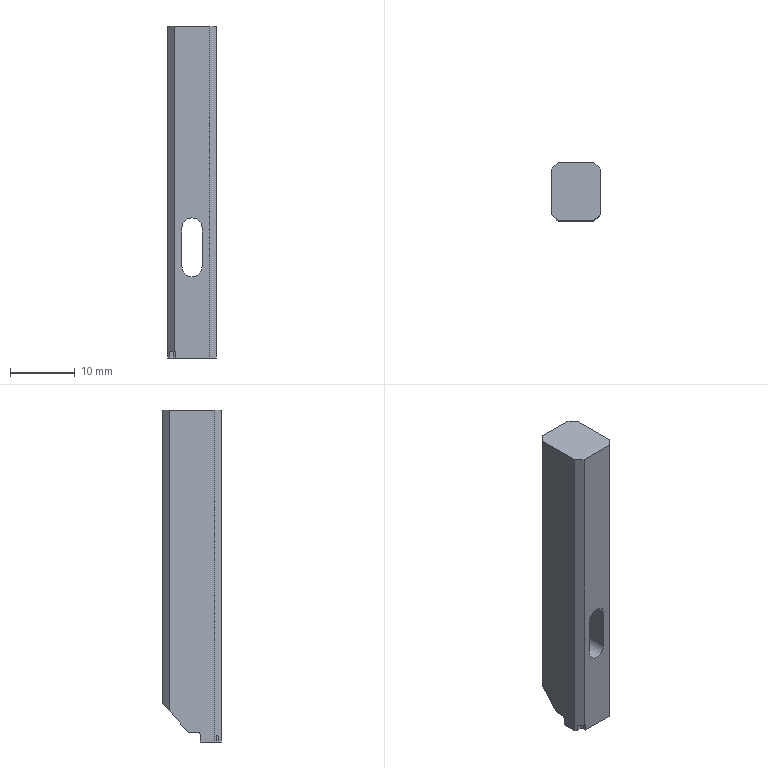Part | STEP file | 03-12 trimming upper-left blade | 1 solid | 23 faces | box 7.5 x 9 x 51.3 mm | volume 2999 mm3 | plane 18 | cylinder 5 | commonest cylinder face diameters 3.1 x3 0.7 x1 1 x1
STEP:
#1=CARTESIAN_POINT('',(3.13,-4.5,21.65));
#2=VERTEX_POINT('',#1);
#3=CARTESIAN_POINT('',(4.68,-4.5,20.1));
#4=VERTEX_POINT('',#3);
#5=CARTESIAN_POINT('',(3.13,-4.5,20.1));
#6=DIRECTION('',(0.,1.,0.));
#7=DIRECTION('',(0.,0.,1.));
#8=AXIS2_PLACEMENT_3D('',#5,#6,#7);
#9=CIRCLE('',#8,1.55);
#10=EDGE_CURVE('',#2,#4,#9,.T.);
#11=ORIENTED_EDGE('',*,*,#10,.F.);
#12=CARTESIAN_POINT('',(3.13,4.5,21.65));
#13=VERTEX_POINT('',#12);
#14=CARTESIAN_POINT('',(3.13,-8.5,21.65));
#15=DIRECTION('',(0.,1.,0.));
#16=VECTOR('',#15,1000.);
#17=LINE('',#14,#16);
#18=EDGE_CURVE('',#2,#13,#17,.T.);
#19=ORIENTED_EDGE('',*,*,#18,.T.);
#20=CARTESIAN_POINT('',(4.68,4.5,20.1));
#21=VERTEX_POINT('',#20);
#22=CARTESIAN_POINT('',(3.13,4.5,20.1));
#23=DIRECTION('',(0.,1.,0.));
#24=DIRECTION('',(0.,0.,1.));
#25=AXIS2_PLACEMENT_3D('',#22,#23,#24);
#26=CIRCLE('',#25,1.55);
#27=EDGE_CURVE('',#13,#21,#26,.T.);
#28=ORIENTED_EDGE('',*,*,#27,.T.);
#29=CARTESIAN_POINT('',(4.68,-8.5,20.1));
#30=DIRECTION('',(0.,1.,0.));
#31=VECTOR('',#30,1000.);
#32=LINE('',#29,#31);
#33=EDGE_CURVE('',#4,#21,#32,.T.);
#34=ORIENTED_EDGE('',*,*,#33,.F.);
#35=EDGE_LOOP('',(#11,#19,#28,#34));
#36=FACE_OUTER_BOUND('',#35,.T.);
#37=CARTESIAN_POINT('',(3.13,-8.5,20.1));
#38=DIRECTION('',(0.,1.,0.));
#39=DIRECTION('',(0.,0.,1.));
#40=AXIS2_PLACEMENT_3D('',#37,#38,#39);
#41=CYLINDRICAL_SURFACE('',#40,1.55);
#42=ADVANCED_FACE('',(#36),#41,.F.);
#43=CARTESIAN_POINT('',(4.68,4.5,14.1));
#44=VERTEX_POINT('',#43);
#45=CARTESIAN_POINT('',(4.68,4.5,20.1));
#46=DIRECTION('',(0.,0.,-1.));
#47=VECTOR('',#46,1000.);
#48=LINE('',#45,#47);
#49=EDGE_CURVE('',#21,#44,#48,.T.);
#50=ORIENTED_EDGE('',*,*,#49,.F.);
#51=ORIENTED_EDGE('',*,*,#27,.F.);
#52=CARTESIAN_POINT('',(1.58,4.5,20.1));
#53=VERTEX_POINT('',#52);
#54=CARTESIAN_POINT('',(3.13,4.5,20.1));
#55=DIRECTION('',(0.,1.,0.));
#56=DIRECTION('',(0.,0.,1.));
#57=AXIS2_PLACEMENT_3D('',#54,#55,#56);
#58=CIRCLE('',#57,1.55);
#59=EDGE_CURVE('',#53,#13,#58,.T.);
#60=ORIENTED_EDGE('',*,*,#59,.F.);
#61=CARTESIAN_POINT('',(1.58,4.5,14.1));
#62=VERTEX_POINT('',#61);
#63=CARTESIAN_POINT('',(1.58,4.5,20.1));
#64=DIRECTION('',(0.,0.,1.));
#65=VECTOR('',#64,1000.);
#66=LINE('',#63,#65);
#67=EDGE_CURVE('',#62,#53,#66,.T.);
#68=ORIENTED_EDGE('',*,*,#67,.F.);
#69=CARTESIAN_POINT('',(3.13,4.5,14.1));
#70=DIRECTION('',(0.,1.,0.));
#71=DIRECTION('',(0.,0.,1.));
#72=AXIS2_PLACEMENT_3D('',#69,#70,#71);
#73=CIRCLE('',#72,1.55);
#74=EDGE_CURVE('',#44,#62,#73,.T.);
#75=ORIENTED_EDGE('',*,*,#74,.F.);
#76=EDGE_LOOP('',(#50,#51,#60,#68,#75));
#77=FACE_BOUND('',#76,.T.);
#78=CARTESIAN_POINT('',(5.88,4.5,6.));
#79=VERTEX_POINT('',#78);
#80=CARTESIAN_POINT('',(0.3804,4.5,6.));
#81=VERTEX_POINT('',#80);
#82=CARTESIAN_POINT('',(7.38,4.5,6.));
#83=DIRECTION('',(-1.,0.,0.));
#84=VECTOR('',#83,1000.);
#85=LINE('',#82,#84);
#86=EDGE_CURVE('',#79,#81,#85,.T.);
#87=ORIENTED_EDGE('',*,*,#86,.T.);
#88=CARTESIAN_POINT('',(0.3804,4.5,51.3));
#89=VERTEX_POINT('',#88);
#90=CARTESIAN_POINT('',(0.3804,4.5,51.3));
#91=DIRECTION('',(0.,0.,1.));
#92=VECTOR('',#91,1000.);
#93=LINE('',#90,#92);
#94=EDGE_CURVE('',#81,#89,#93,.T.);
#95=ORIENTED_EDGE('',*,*,#94,.T.);
#96=CARTESIAN_POINT('',(5.88,4.5,51.3));
#97=VERTEX_POINT('',#96);
#98=CARTESIAN_POINT('',(-6.,4.5,51.3));
#99=DIRECTION('',(-1.,0.,0.));
#100=VECTOR('',#99,1000.);
#101=LINE('',#98,#100);
#102=EDGE_CURVE('',#97,#89,#101,.T.);
#103=ORIENTED_EDGE('',*,*,#102,.F.);
#104=CARTESIAN_POINT('',(5.88,4.5,51.3));
#105=DIRECTION('',(0.,0.,-1.));
#106=VECTOR('',#105,1000.);
#107=LINE('',#104,#106);
#108=EDGE_CURVE('',#97,#79,#107,.T.);
#109=ORIENTED_EDGE('',*,*,#108,.T.);
#110=EDGE_LOOP('',(#87,#95,#103,#109));
#111=FACE_OUTER_BOUND('',#110,.T.);
#112=CARTESIAN_POINT('',(-6.,4.5,51.3));
#113=DIRECTION('',(0.,-1.,0.));
#114=DIRECTION('',(0.,0.,-1.));
#115=AXIS2_PLACEMENT_3D('',#112,#113,#114);
#116=PLANE('',#115);
#117=ADVANCED_FACE('',(#77,#111),#116,.F.);
#118=CARTESIAN_POINT('',(1.58,-4.5,14.1));
#119=VERTEX_POINT('',#118);
#120=CARTESIAN_POINT('',(1.58,-4.5,20.1));
#121=VERTEX_POINT('',#120);
#122=CARTESIAN_POINT('',(1.58,-4.5,51.3));
#123=DIRECTION('',(0.,0.,1.));
#124=VECTOR('',#123,1000.);
#125=LINE('',#122,#124);
#126=EDGE_CURVE('',#119,#121,#125,.T.);
#127=ORIENTED_EDGE('',*,*,#126,.T.);
#128=CARTESIAN_POINT('',(3.13,-4.5,20.1));
#129=DIRECTION('',(0.,1.,0.));
#130=DIRECTION('',(0.,0.,1.));
#131=AXIS2_PLACEMENT_3D('',#128,#129,#130);
#132=CIRCLE('',#131,1.55);
#133=EDGE_CURVE('',#121,#2,#132,.T.);
#134=ORIENTED_EDGE('',*,*,#133,.T.);
#135=ORIENTED_EDGE('',*,*,#10,.T.);
#136=CARTESIAN_POINT('',(4.68,-4.5,14.1));
#137=VERTEX_POINT('',#136);
#138=CARTESIAN_POINT('',(4.68,-4.5,51.3));
#139=DIRECTION('',(0.,0.,-1.));
#140=VECTOR('',#139,1000.);
#141=LINE('',#138,#140);
#142=EDGE_CURVE('',#4,#137,#141,.T.);
#143=ORIENTED_EDGE('',*,*,#142,.T.);
#144=CARTESIAN_POINT('',(3.13,-4.5,14.1));
#145=DIRECTION('',(0.,1.,0.));
#146=DIRECTION('',(0.,0.,1.));
#147=AXIS2_PLACEMENT_3D('',#144,#145,#146);
#148=CIRCLE('',#147,1.55);
#149=EDGE_CURVE('',#137,#119,#148,.T.);
#150=ORIENTED_EDGE('',*,*,#149,.T.);
#151=EDGE_LOOP('',(#127,#134,#135,#143,#150));
#152=FACE_BOUND('',#151,.T.);
#153=CARTESIAN_POINT('',(0.6304,-4.5,1.));
#154=VERTEX_POINT('',#153);
#155=CARTESIAN_POINT('',(0.3804,-4.5,1.));
#156=VERTEX_POINT('',#155);
#157=CARTESIAN_POINT('',(-6.,-4.5,1.));
#158=DIRECTION('',(-1.,0.,0.));
#159=VECTOR('',#158,1000.);
#160=LINE('',#157,#159);
#161=EDGE_CURVE('',#154,#156,#160,.T.);
#162=ORIENTED_EDGE('',*,*,#161,.F.);
#163=CARTESIAN_POINT('',(0.6304,-4.5,0.));
#164=VERTEX_POINT('',#163);
#165=CARTESIAN_POINT('',(0.6304,-4.5,51.3));
#166=DIRECTION('',(0.,0.,-1.));
#167=VECTOR('',#166,1000.);
#168=LINE('',#165,#167);
#169=EDGE_CURVE('',#154,#164,#168,.T.);
#170=ORIENTED_EDGE('',*,*,#169,.T.);
#171=CARTESIAN_POINT('',(5.88,-4.5,0.));
#172=VERTEX_POINT('',#171);
#173=CARTESIAN_POINT('',(-6.,-4.5,0.));
#174=DIRECTION('',(1.,0.,0.));
#175=VECTOR('',#174,1000.);
#176=LINE('',#173,#175);
#177=EDGE_CURVE('',#164,#172,#176,.T.);
#178=ORIENTED_EDGE('',*,*,#177,.T.);
#179=CARTESIAN_POINT('',(5.88,-4.5,51.3));
#180=VERTEX_POINT('',#179);
#181=CARTESIAN_POINT('',(5.88,-4.5,51.3));
#182=DIRECTION('',(0.,0.,1.));
#183=VECTOR('',#182,1000.);
#184=LINE('',#181,#183);
#185=EDGE_CURVE('',#172,#180,#184,.T.);
#186=ORIENTED_EDGE('',*,*,#185,.T.);
#187=CARTESIAN_POINT('',(0.3804,-4.5,51.3));
#188=VERTEX_POINT('',#187);
#189=CARTESIAN_POINT('',(-6.,-4.5,51.3));
#190=DIRECTION('',(1.,0.,0.));
#191=VECTOR('',#190,1000.);
#192=LINE('',#189,#191);
#193=EDGE_CURVE('',#188,#180,#192,.T.);
#194=ORIENTED_EDGE('',*,*,#193,.F.);
#195=CARTESIAN_POINT('',(0.3804,-4.5,51.3));
#196=DIRECTION('',(0.,0.,-1.));
#197=VECTOR('',#196,1000.);
#198=LINE('',#195,#197);
#199=EDGE_CURVE('',#188,#156,#198,.T.);
#200=ORIENTED_EDGE('',*,*,#199,.T.);
#201=EDGE_LOOP('',(#162,#170,#178,#186,#194,#200));
#202=FACE_OUTER_BOUND('',#201,.T.);
#203=CARTESIAN_POINT('',(-6.,-4.5,51.3));
#204=DIRECTION('',(0.,1.,0.));
#205=DIRECTION('',(0.,0.,1.));
#206=AXIS2_PLACEMENT_3D('',#203,#204,#205);
#207=PLANE('',#206);
#208=ADVANCED_FACE('',(#152,#202),#207,.F.);
#209=CARTESIAN_POINT('',(-0.6196,-3.5,51.3));
#210=VERTEX_POINT('',#209);
#211=CARTESIAN_POINT('',(-0.6196,3.5,51.3));
#212=VERTEX_POINT('',#211);
#213=CARTESIAN_POINT('',(-0.6196,-4.5,51.3));
#214=DIRECTION('',(0.,1.,0.));
#215=VECTOR('',#214,1000.);
#216=LINE('',#213,#215);
#217=EDGE_CURVE('',#210,#212,#216,.T.);
#218=ORIENTED_EDGE('',*,*,#217,.F.);
#219=CARTESIAN_POINT('',(3.19,-7.31,51.3));
#220=DIRECTION('',(0.7071,-0.7071,0.));
#221=VECTOR('',#220,1000.);
#222=LINE('',#219,#221);
#223=EDGE_CURVE('',#210,#188,#222,.T.);
#224=ORIENTED_EDGE('',*,*,#223,.T.);
#225=ORIENTED_EDGE('',*,*,#193,.T.);
#226=CARTESIAN_POINT('',(6.88,-3.5,51.3));
#227=VERTEX_POINT('',#226);
#228=CARTESIAN_POINT('',(5.94,-4.44,51.3));
#229=DIRECTION('',(0.7071,0.7071,0.));
#230=VECTOR('',#229,1000.);
#231=LINE('',#228,#230);
#232=EDGE_CURVE('',#180,#227,#231,.T.);
#233=ORIENTED_EDGE('',*,*,#232,.T.);
#234=CARTESIAN_POINT('',(6.88,3.5,51.3));
#235=VERTEX_POINT('',#234);
#236=CARTESIAN_POINT('',(6.88,-4.5,51.3));
#237=DIRECTION('',(0.,-1.,0.));
#238=VECTOR('',#237,1000.);
#239=LINE('',#236,#238);
#240=EDGE_CURVE('',#235,#227,#239,.T.);
#241=ORIENTED_EDGE('',*,*,#240,.F.);
#242=CARTESIAN_POINT('',(10.44,-0.05981,51.3));
#243=DIRECTION('',(-0.7071,0.7071,0.));
#244=VECTOR('',#243,1000.);
#245=LINE('',#242,#244);
#246=EDGE_CURVE('',#235,#97,#245,.T.);
#247=ORIENTED_EDGE('',*,*,#246,.T.);
#248=ORIENTED_EDGE('',*,*,#102,.T.);
#249=CARTESIAN_POINT('',(-1.31,2.81,51.3));
#250=DIRECTION('',(-0.7071,-0.7071,0.));
#251=VECTOR('',#250,1000.);
#252=LINE('',#249,#251);
#253=EDGE_CURVE('',#89,#212,#252,.T.);
#254=ORIENTED_EDGE('',*,*,#253,.T.);
#255=EDGE_LOOP('',(#218,#224,#225,#233,#241,#247,#248,#254));
#256=FACE_OUTER_BOUND('',#255,.T.);
#257=CARTESIAN_POINT('',(6.,-4.5,51.3));
#258=DIRECTION('',(0.,0.,1.));
#259=DIRECTION('',(1.,0.,0.));
#260=AXIS2_PLACEMENT_3D('',#257,#258,#259);
#261=PLANE('',#260);
#262=ADVANCED_FACE('',(#256),#261,.T.);
#263=CARTESIAN_POINT('',(0.2804,-3.75,0.));
#264=VERTEX_POINT('',#263);
#265=CARTESIAN_POINT('',(0.6304,-4.1,0.));
#266=VERTEX_POINT('',#265);
#267=CARTESIAN_POINT('',(0.2804,-4.1,0.));
#268=DIRECTION('',(0.,0.,-1.));
#269=DIRECTION('',(-1.,0.,0.));
#270=AXIS2_PLACEMENT_3D('',#267,#268,#269);
#271=CIRCLE('',#270,0.35);
#272=EDGE_CURVE('',#264,#266,#271,.T.);
#273=ORIENTED_EDGE('',*,*,#272,.F.);
#274=CARTESIAN_POINT('',(-0.3696,-3.75,0.));
#275=VERTEX_POINT('',#274);
#276=CARTESIAN_POINT('',(0.2804,-3.75,0.));
#277=DIRECTION('',(1.,0.,0.));
#278=VECTOR('',#277,1000.);
#279=LINE('',#276,#278);
#280=EDGE_CURVE('',#275,#264,#279,.T.);
#281=ORIENTED_EDGE('',*,*,#280,.F.);
#282=CARTESIAN_POINT('',(-0.6196,-3.5,0.));
#283=VERTEX_POINT('',#282);
#284=CARTESIAN_POINT('',(0.3804,-4.5,0.));
#285=DIRECTION('',(-0.7071,0.7071,0.));
#286=VECTOR('',#285,1000.);
#287=LINE('',#284,#286);
#288=EDGE_CURVE('',#275,#283,#287,.T.);
#289=ORIENTED_EDGE('',*,*,#288,.T.);
#290=CARTESIAN_POINT('',(-0.6196,-1.3,0.));
#291=VERTEX_POINT('',#290);
#292=CARTESIAN_POINT('',(-0.6196,4.5,0.));
#293=DIRECTION('',(0.,-1.,0.));
#294=VECTOR('',#293,1000.);
#295=LINE('',#292,#294);
#296=EDGE_CURVE('',#291,#283,#295,.T.);
#297=ORIENTED_EDGE('',*,*,#296,.F.);
#298=CARTESIAN_POINT('',(6.88,-1.3,0.));
#299=VERTEX_POINT('',#298);
#300=CARTESIAN_POINT('',(6.,-1.3,0.));
#301=DIRECTION('',(1.,0.,0.));
#302=VECTOR('',#301,1000.);
#303=LINE('',#300,#302);
#304=EDGE_CURVE('',#291,#299,#303,.T.);
#305=ORIENTED_EDGE('',*,*,#304,.T.);
#306=CARTESIAN_POINT('',(6.88,-3.5,0.));
#307=VERTEX_POINT('',#306);
#308=CARTESIAN_POINT('',(6.88,4.815,0.));
#309=DIRECTION('',(0.,1.,0.));
#310=VECTOR('',#309,1000.);
#311=LINE('',#308,#310);
#312=EDGE_CURVE('',#307,#299,#311,.T.);
#313=ORIENTED_EDGE('',*,*,#312,.F.);
#314=CARTESIAN_POINT('',(5.88,-4.5,0.));
#315=DIRECTION('',(-0.7071,-0.7071,0.));
#316=VECTOR('',#315,1000.);
#317=LINE('',#314,#316);
#318=EDGE_CURVE('',#307,#172,#317,.T.);
#319=ORIENTED_EDGE('',*,*,#318,.T.);
#320=ORIENTED_EDGE('',*,*,#177,.F.);
#321=CARTESIAN_POINT('',(0.6304,-4.1,0.));
#322=DIRECTION('',(0.,-1.,0.));
#323=VECTOR('',#322,1000.);
#324=LINE('',#321,#323);
#325=EDGE_CURVE('',#266,#164,#324,.T.);
#326=ORIENTED_EDGE('',*,*,#325,.F.);
#327=EDGE_LOOP('',(#273,#281,#289,#297,#305,#313,#319,#320,#326));
#328=FACE_OUTER_BOUND('',#327,.T.);
#329=CARTESIAN_POINT('',(6.,-4.5,0.));
#330=DIRECTION('',(0.,0.,1.));
#331=DIRECTION('',(1.,0.,0.));
#332=AXIS2_PLACEMENT_3D('',#329,#330,#331);
#333=PLANE('',#332);
#334=ADVANCED_FACE('',(#328),#333,.F.);
#335=ORIENTED_EDGE('',*,*,#296,.T.);
#336=CARTESIAN_POINT('',(-0.6196,-3.5,6.));
#337=DIRECTION('',(0.,0.,1.));
#338=VECTOR('',#337,1000.);
#339=LINE('',#336,#338);
#340=EDGE_CURVE('',#283,#210,#339,.T.);
#341=ORIENTED_EDGE('',*,*,#340,.T.);
#342=ORIENTED_EDGE('',*,*,#217,.T.);
#343=CARTESIAN_POINT('',(-0.6196,3.5,4.846));
#344=VERTEX_POINT('',#343);
#345=CARTESIAN_POINT('',(-0.6196,3.5,6.));
#346=DIRECTION('',(0.,0.,-1.));
#347=VECTOR('',#346,1000.);
#348=LINE('',#345,#347);
#349=EDGE_CURVE('',#212,#344,#348,.T.);
#350=ORIENTED_EDGE('',*,*,#349,.T.);
#351=CARTESIAN_POINT('',(-0.6196,0.6,1.5));
#352=VERTEX_POINT('',#351);
#353=CARTESIAN_POINT('',(-0.6196,-0.7,0.));
#354=DIRECTION('',(0.,0.6549,0.7557));
#355=VECTOR('',#354,1000.);
#356=LINE('',#353,#355);
#357=EDGE_CURVE('',#352,#344,#356,.T.);
#358=ORIENTED_EDGE('',*,*,#357,.F.);
#359=CARTESIAN_POINT('',(-0.6196,-0.8,1.5));
#360=VERTEX_POINT('',#359);
#361=CARTESIAN_POINT('',(-0.6196,1.172,1.5));
#362=DIRECTION('',(0.,1.,0.));
#363=VECTOR('',#362,1000.);
#364=LINE('',#361,#363);
#365=EDGE_CURVE('',#360,#352,#364,.T.);
#366=ORIENTED_EDGE('',*,*,#365,.F.);
#367=CARTESIAN_POINT('',(-0.6196,-1.3,1.));
#368=VERTEX_POINT('',#367);
#369=CARTESIAN_POINT('',(-0.6196,-0.8,1.));
#370=DIRECTION('',(-1.,0.,0.));
#371=DIRECTION('',(0.,1.,0.));
#372=AXIS2_PLACEMENT_3D('',#369,#370,#371);
#373=CIRCLE('',#372,0.5);
#374=EDGE_CURVE('',#368,#360,#373,.T.);
#375=ORIENTED_EDGE('',*,*,#374,.F.);
#376=CARTESIAN_POINT('',(-0.6196,-1.3,-0.1478));
#377=DIRECTION('',(0.,0.,1.));
#378=VECTOR('',#377,1000.);
#379=LINE('',#376,#378);
#380=EDGE_CURVE('',#291,#368,#379,.T.);
#381=ORIENTED_EDGE('',*,*,#380,.F.);
#382=EDGE_LOOP('',(#335,#341,#342,#350,#358,#366,#375,#381));
#383=FACE_OUTER_BOUND('',#382,.T.);
#384=CARTESIAN_POINT('',(-0.6196,4.5,6.));
#385=DIRECTION('',(1.,0.,0.));
#386=DIRECTION('',(0.,1.,0.));
#387=AXIS2_PLACEMENT_3D('',#384,#385,#386);
#388=PLANE('',#387);
#389=ADVANCED_FACE('',(#383),#388,.F.);
#390=ORIENTED_EDGE('',*,*,#357,.T.);
#391=CARTESIAN_POINT('',(-0.22,3.9,5.307));
#392=DIRECTION('',(0.5479,0.5479,0.6322));
#393=VECTOR('',#392,1000.);
#394=LINE('',#391,#393);
#395=EDGE_CURVE('',#344,#81,#394,.T.);
#396=ORIENTED_EDGE('',*,*,#395,.T.);
#397=ORIENTED_EDGE('',*,*,#86,.F.);
#398=CARTESIAN_POINT('',(6.88,3.5,4.846));
#399=VERTEX_POINT('',#398);
#400=CARTESIAN_POINT('',(-9.81,20.19,24.104));
#401=DIRECTION('',(0.5479,-0.5479,-0.6322));
#402=VECTOR('',#401,1000.);
#403=LINE('',#400,#402);
#404=EDGE_CURVE('',#79,#399,#403,.T.);
#405=ORIENTED_EDGE('',*,*,#404,.T.);
#406=CARTESIAN_POINT('',(6.88,0.6,1.5));
#407=VERTEX_POINT('',#406);
#408=CARTESIAN_POINT('',(6.88,-0.7,0.));
#409=DIRECTION('',(0.,-0.6549,-0.7557));
#410=VECTOR('',#409,1000.);
#411=LINE('',#408,#410);
#412=EDGE_CURVE('',#399,#407,#411,.T.);
#413=ORIENTED_EDGE('',*,*,#412,.T.);
#414=CARTESIAN_POINT('',(7.38,0.6,1.5));
#415=DIRECTION('',(-1.,0.,0.));
#416=VECTOR('',#415,1000.);
#417=LINE('',#414,#416);
#418=EDGE_CURVE('',#407,#352,#417,.T.);
#419=ORIENTED_EDGE('',*,*,#418,.T.);
#420=EDGE_LOOP('',(#390,#396,#397,#405,#413,#419));
#421=FACE_OUTER_BOUND('',#420,.T.);
#422=CARTESIAN_POINT('',(7.38,-0.7,0.));
#423=DIRECTION('',(0.,-0.7557,0.6549));
#424=DIRECTION('',(0.,-0.6549,-0.7557));
#425=AXIS2_PLACEMENT_3D('',#422,#423,#424);
#426=PLANE('',#425);
#427=ADVANCED_FACE('',(#421),#426,.F.);
#428=CARTESIAN_POINT('',(6.88,-0.8,1.5));
#429=VERTEX_POINT('',#428);
#430=CARTESIAN_POINT('',(6.38,-0.8,1.5));
#431=DIRECTION('',(-1.,0.,0.));
#432=VECTOR('',#431,1000.);
#433=LINE('',#430,#432);
#434=EDGE_CURVE('',#429,#360,#433,.T.);
#435=ORIENTED_EDGE('',*,*,#434,.F.);
#436=CARTESIAN_POINT('',(6.88,-1.3,1.));
#437=VERTEX_POINT('',#436);
#438=CARTESIAN_POINT('',(6.88,-0.8,1.));
#439=DIRECTION('',(1.,0.,0.));
#440=DIRECTION('',(0.,-1.,0.));
#441=AXIS2_PLACEMENT_3D('',#438,#439,#440);
#442=CIRCLE('',#441,0.5);
#443=EDGE_CURVE('',#429,#437,#442,.T.);
#444=ORIENTED_EDGE('',*,*,#443,.T.);
#445=CARTESIAN_POINT('',(6.38,-1.3,1.));
#446=DIRECTION('',(-1.,0.,0.));
#447=VECTOR('',#446,1000.);
#448=LINE('',#445,#447);
#449=EDGE_CURVE('',#437,#368,#448,.T.);
#450=ORIENTED_EDGE('',*,*,#449,.T.);
#451=ORIENTED_EDGE('',*,*,#374,.T.);
#452=EDGE_LOOP('',(#435,#444,#450,#451));
#453=FACE_OUTER_BOUND('',#452,.T.);
#454=CARTESIAN_POINT('',(6.38,-0.8,1.));
#455=DIRECTION('',(-1.,0.,0.));
#456=DIRECTION('',(0.,-1.,0.));
#457=AXIS2_PLACEMENT_3D('',#454,#455,#456);
#458=CYLINDRICAL_SURFACE('',#457,0.5);
#459=ADVANCED_FACE('',(#453),#458,.F.);
#460=ORIENTED_EDGE('',*,*,#449,.F.);
#461=CARTESIAN_POINT('',(6.88,-1.3,-0.1478));
#462=DIRECTION('',(0.,0.,-1.));
#463=VECTOR('',#462,1000.);
#464=LINE('',#461,#463);
#465=EDGE_CURVE('',#437,#299,#464,.T.);
#466=ORIENTED_EDGE('',*,*,#465,.T.);
#467=ORIENTED_EDGE('',*,*,#304,.F.);
#468=ORIENTED_EDGE('',*,*,#380,.T.);
#469=EDGE_LOOP('',(#460,#466,#467,#468));
#470=FACE_OUTER_BOUND('',#469,.T.);
#471=CARTESIAN_POINT('',(6.38,-1.3,-0.1478));
#472=DIRECTION('',(0.,-1.,0.));
#473=DIRECTION('',(1.,0.,0.));
#474=AXIS2_PLACEMENT_3D('',#471,#472,#473);
#475=PLANE('',#474);
#476=ADVANCED_FACE('',(#470),#475,.F.);
#477=ORIENTED_EDGE('',*,*,#418,.F.);
#478=CARTESIAN_POINT('',(6.88,1.172,1.5));
#479=DIRECTION('',(0.,-1.,0.));
#480=VECTOR('',#479,1000.);
#481=LINE('',#478,#480);
#482=EDGE_CURVE('',#407,#429,#481,.T.);
#483=ORIENTED_EDGE('',*,*,#482,.T.);
#484=ORIENTED_EDGE('',*,*,#434,.T.);
#485=ORIENTED_EDGE('',*,*,#365,.T.);
#486=EDGE_LOOP('',(#477,#483,#484,#485));
#487=FACE_OUTER_BOUND('',#486,.T.);
#488=CARTESIAN_POINT('',(6.38,1.172,1.5));
#489=DIRECTION('',(0.,0.,1.));
#490=DIRECTION('',(0.,-1.,0.));
#491=AXIS2_PLACEMENT_3D('',#488,#489,#490);
#492=PLANE('',#491);
#493=ADVANCED_FACE('',(#487),#492,.F.);
#494=ORIENTED_EDGE('',*,*,#412,.F.);
#495=CARTESIAN_POINT('',(6.88,3.5,63.));
#496=DIRECTION('',(0.,0.,1.));
#497=VECTOR('',#496,1000.);
#498=LINE('',#495,#497);
#499=EDGE_CURVE('',#399,#235,#498,.T.);
#500=ORIENTED_EDGE('',*,*,#499,.T.);
#501=ORIENTED_EDGE('',*,*,#240,.T.);
#502=CARTESIAN_POINT('',(6.88,-3.5,63.));
#503=DIRECTION('',(0.,0.,-1.));
#504=VECTOR('',#503,1000.);
#505=LINE('',#502,#504);
#506=EDGE_CURVE('',#227,#307,#505,.T.);
#507=ORIENTED_EDGE('',*,*,#506,.T.);
#508=ORIENTED_EDGE('',*,*,#312,.T.);
#509=ORIENTED_EDGE('',*,*,#465,.F.);
#510=ORIENTED_EDGE('',*,*,#443,.F.);
#511=ORIENTED_EDGE('',*,*,#482,.F.);
#512=EDGE_LOOP('',(#494,#500,#501,#507,#508,#509,#510,#511));
#513=FACE_OUTER_BOUND('',#512,.T.);
#514=CARTESIAN_POINT('',(6.88,4.815,63.));
#515=DIRECTION('',(-1.,0.,0.));
#516=DIRECTION('',(0.,-1.,0.));
#517=AXIS2_PLACEMENT_3D('',#514,#515,#516);
#518=PLANE('',#517);
#519=ADVANCED_FACE('',(#513),#518,.F.);
#520=CARTESIAN_POINT('',(-0.3696,-3.75,1.));
#521=VERTEX_POINT('',#520);
#522=CARTESIAN_POINT('',(-0.3696,-3.75,51.3));
#523=DIRECTION('',(0.,0.,-1.));
#524=VECTOR('',#523,1000.);
#525=LINE('',#522,#524);
#526=EDGE_CURVE('',#521,#275,#525,.T.);
#527=ORIENTED_EDGE('',*,*,#526,.F.);
#528=CARTESIAN_POINT('',(0.3804,-4.5,1.));
#529=DIRECTION('',(0.7071,-0.7071,0.));
#530=VECTOR('',#529,1000.);
#531=LINE('',#528,#530);
#532=EDGE_CURVE('',#521,#156,#531,.T.);
#533=ORIENTED_EDGE('',*,*,#532,.T.);
#534=ORIENTED_EDGE('',*,*,#199,.F.);
#535=ORIENTED_EDGE('',*,*,#223,.F.);
#536=ORIENTED_EDGE('',*,*,#340,.F.);
#537=ORIENTED_EDGE('',*,*,#288,.F.);
#538=EDGE_LOOP('',(#527,#533,#534,#535,#536,#537));
#539=FACE_OUTER_BOUND('',#538,.T.);
#540=CARTESIAN_POINT('',(0.3804,-4.5,51.3));
#541=DIRECTION('',(0.7071,0.7071,0.));
#542=DIRECTION('',(-0.7071,0.7071,0.));
#543=AXIS2_PLACEMENT_3D('',#540,#541,#542);
#544=PLANE('',#543);
#545=ADVANCED_FACE('',(#539),#544,.F.);
#546=ORIENTED_EDGE('',*,*,#253,.F.);
#547=ORIENTED_EDGE('',*,*,#94,.F.);
#548=ORIENTED_EDGE('',*,*,#395,.F.);
#549=ORIENTED_EDGE('',*,*,#349,.F.);
#550=EDGE_LOOP('',(#546,#547,#548,#549));
#551=FACE_OUTER_BOUND('',#550,.T.);
#552=CARTESIAN_POINT('',(-0.6196,3.5,6.));
#553=DIRECTION('',(0.7071,-0.7071,0.));
#554=DIRECTION('',(0.7071,0.7071,0.));
#555=AXIS2_PLACEMENT_3D('',#552,#553,#554);
#556=PLANE('',#555);
#557=ADVANCED_FACE('',(#551),#556,.F.);
#558=ORIENTED_EDGE('',*,*,#246,.F.);
#559=ORIENTED_EDGE('',*,*,#499,.F.);
#560=ORIENTED_EDGE('',*,*,#404,.F.);
#561=ORIENTED_EDGE('',*,*,#108,.F.);
#562=EDGE_LOOP('',(#558,#559,#560,#561));
#563=FACE_OUTER_BOUND('',#562,.T.);
#564=CARTESIAN_POINT('',(5.88,4.5,51.3));
#565=DIRECTION('',(-0.7071,-0.7071,0.));
#566=DIRECTION('',(0.7071,-0.7071,0.));
#567=AXIS2_PLACEMENT_3D('',#564,#565,#566);
#568=PLANE('',#567);
#569=ADVANCED_FACE('',(#563),#568,.F.);
#570=ORIENTED_EDGE('',*,*,#318,.F.);
#571=ORIENTED_EDGE('',*,*,#506,.F.);
#572=ORIENTED_EDGE('',*,*,#232,.F.);
#573=ORIENTED_EDGE('',*,*,#185,.F.);
#574=EDGE_LOOP('',(#570,#571,#572,#573));
#575=FACE_OUTER_BOUND('',#574,.T.);
#576=CARTESIAN_POINT('',(5.88,-4.5,51.3));
#577=DIRECTION('',(-0.7071,0.7071,0.));
#578=DIRECTION('',(-0.7071,-0.7071,0.));
#579=AXIS2_PLACEMENT_3D('',#576,#577,#578);
#580=PLANE('',#579);
#581=ADVANCED_FACE('',(#575),#580,.F.);
#582=ORIENTED_EDGE('',*,*,#18,.F.);
#583=ORIENTED_EDGE('',*,*,#133,.F.);
#584=CARTESIAN_POINT('',(1.58,-8.5,20.1));
#585=DIRECTION('',(0.,1.,0.));
#586=VECTOR('',#585,1000.);
#587=LINE('',#584,#586);
#588=EDGE_CURVE('',#121,#53,#587,.T.);
#589=ORIENTED_EDGE('',*,*,#588,.T.);
#590=ORIENTED_EDGE('',*,*,#59,.T.);
#591=EDGE_LOOP('',(#582,#583,#589,#590));
#592=FACE_OUTER_BOUND('',#591,.T.);
#593=CARTESIAN_POINT('',(3.13,-8.5,20.1));
#594=DIRECTION('',(0.,1.,0.));
#595=DIRECTION('',(0.,0.,1.));
#596=AXIS2_PLACEMENT_3D('',#593,#594,#595);
#597=CYLINDRICAL_SURFACE('',#596,1.55);
#598=ADVANCED_FACE('',(#592),#597,.F.);
#599=CARTESIAN_POINT('',(1.58,-8.5,14.1));
#600=DIRECTION('',(0.,1.,0.));
#601=VECTOR('',#600,1000.);
#602=LINE('',#599,#601);
#603=EDGE_CURVE('',#119,#62,#602,.T.);
#604=ORIENTED_EDGE('',*,*,#603,.T.);
#605=ORIENTED_EDGE('',*,*,#67,.T.);
#606=ORIENTED_EDGE('',*,*,#588,.F.);
#607=ORIENTED_EDGE('',*,*,#126,.F.);
#608=EDGE_LOOP('',(#604,#605,#606,#607));
#609=FACE_OUTER_BOUND('',#608,.T.);
#610=CARTESIAN_POINT('',(1.58,-8.5,20.1));
#611=DIRECTION('',(-1.,0.,0.));
#612=DIRECTION('',(0.,0.,1.));
#613=AXIS2_PLACEMENT_3D('',#610,#611,#612);
#614=PLANE('',#613);
#615=ADVANCED_FACE('',(#609),#614,.F.);
#616=CARTESIAN_POINT('',(4.68,-8.5,14.1));
#617=DIRECTION('',(0.,1.,0.));
#618=VECTOR('',#617,1000.);
#619=LINE('',#616,#618);
#620=EDGE_CURVE('',#137,#44,#619,.T.);
#621=ORIENTED_EDGE('',*,*,#620,.T.);
#622=ORIENTED_EDGE('',*,*,#74,.T.);
#623=ORIENTED_EDGE('',*,*,#603,.F.);
#624=ORIENTED_EDGE('',*,*,#149,.F.);
#625=EDGE_LOOP('',(#621,#622,#623,#624));
#626=FACE_OUTER_BOUND('',#625,.T.);
#627=CARTESIAN_POINT('',(3.13,-8.5,14.1));
#628=DIRECTION('',(0.,1.,0.));
#629=DIRECTION('',(0.,0.,1.));
#630=AXIS2_PLACEMENT_3D('',#627,#628,#629);
#631=CYLINDRICAL_SURFACE('',#630,1.55);
#632=ADVANCED_FACE('',(#626),#631,.F.);
#633=ORIENTED_EDGE('',*,*,#33,.T.);
#634=ORIENTED_EDGE('',*,*,#49,.T.);
#635=ORIENTED_EDGE('',*,*,#620,.F.);
#636=ORIENTED_EDGE('',*,*,#142,.F.);
#637=EDGE_LOOP('',(#633,#634,#635,#636));
#638=FACE_OUTER_BOUND('',#637,.T.);
#639=CARTESIAN_POINT('',(4.68,-8.5,20.1));
#640=DIRECTION('',(1.,0.,0.));
#641=DIRECTION('',(0.,0.,-1.));
#642=AXIS2_PLACEMENT_3D('',#639,#640,#641);
#643=PLANE('',#642);
#644=ADVANCED_FACE('',(#638),#643,.F.);
#645=CARTESIAN_POINT('',(0.6304,-4.1,1.));
#646=VERTEX_POINT('',#645);
#647=CARTESIAN_POINT('',(0.6304,-4.1,1.));
#648=DIRECTION('',(0.,-1.,0.));
#649=VECTOR('',#648,1000.);
#650=LINE('',#647,#649);
#651=EDGE_CURVE('',#646,#154,#650,.T.);
#652=ORIENTED_EDGE('',*,*,#651,.F.);
#653=CARTESIAN_POINT('',(0.6304,-4.1,1.));
#654=DIRECTION('',(0.,0.,-1.));
#655=VECTOR('',#654,1000.);
#656=LINE('',#653,#655);
#657=EDGE_CURVE('',#646,#266,#656,.T.);
#658=ORIENTED_EDGE('',*,*,#657,.T.);
#659=ORIENTED_EDGE('',*,*,#325,.T.);
#660=ORIENTED_EDGE('',*,*,#169,.F.);
#661=EDGE_LOOP('',(#652,#658,#659,#660));
#662=FACE_OUTER_BOUND('',#661,.T.);
#663=CARTESIAN_POINT('',(0.6304,-4.1,1.));
#664=DIRECTION('',(1.,0.,0.));
#665=DIRECTION('',(0.,0.,-1.));
#666=AXIS2_PLACEMENT_3D('',#663,#664,#665);
#667=PLANE('',#666);
#668=ADVANCED_FACE('',(#662),#667,.F.);
#669=ORIENTED_EDGE('',*,*,#161,.T.);
#670=ORIENTED_EDGE('',*,*,#532,.F.);
#671=CARTESIAN_POINT('',(0.2804,-3.75,1.));
#672=VERTEX_POINT('',#671);
#673=CARTESIAN_POINT('',(0.2804,-3.75,1.));
#674=DIRECTION('',(1.,0.,0.));
#675=VECTOR('',#674,1000.);
#676=LINE('',#673,#675);
#677=EDGE_CURVE('',#521,#672,#676,.T.);
#678=ORIENTED_EDGE('',*,*,#677,.T.);
#679=CARTESIAN_POINT('',(0.2804,-4.1,1.));
#680=DIRECTION('',(0.,0.,-1.));
#681=DIRECTION('',(-1.,0.,0.));
#682=AXIS2_PLACEMENT_3D('',#679,#680,#681);
#683=CIRCLE('',#682,0.35);
#684=EDGE_CURVE('',#672,#646,#683,.T.);
#685=ORIENTED_EDGE('',*,*,#684,.T.);
#686=ORIENTED_EDGE('',*,*,#651,.T.);
#687=EDGE_LOOP('',(#669,#670,#678,#685,#686));
#688=FACE_OUTER_BOUND('',#687,.T.);
#689=CARTESIAN_POINT('',(0.2804,-4.1,1.));
#690=DIRECTION('',(0.,0.,-1.));
#691=DIRECTION('',(-1.,0.,0.));
#692=AXIS2_PLACEMENT_3D('',#689,#690,#691);
#693=PLANE('',#692);
#694=ADVANCED_FACE('',(#688),#693,.T.);
#695=ORIENTED_EDGE('',*,*,#272,.T.);
#696=ORIENTED_EDGE('',*,*,#657,.F.);
#697=ORIENTED_EDGE('',*,*,#684,.F.);
#698=CARTESIAN_POINT('',(0.2804,-3.75,1.));
#699=DIRECTION('',(0.,0.,-1.));
#700=VECTOR('',#699,1000.);
#701=LINE('',#698,#700);
#702=EDGE_CURVE('',#672,#264,#701,.T.);
#703=ORIENTED_EDGE('',*,*,#702,.T.);
#704=EDGE_LOOP('',(#695,#696,#697,#703));
#705=FACE_OUTER_BOUND('',#704,.T.);
#706=CARTESIAN_POINT('',(0.2804,-4.1,1.));
#707=DIRECTION('',(0.,0.,-1.));
#708=DIRECTION('',(-1.,0.,0.));
#709=AXIS2_PLACEMENT_3D('',#706,#707,#708);
#710=CYLINDRICAL_SURFACE('',#709,0.35);
#711=ADVANCED_FACE('',(#705),#710,.F.);
#712=ORIENTED_EDGE('',*,*,#526,.T.);
#713=ORIENTED_EDGE('',*,*,#280,.T.);
#714=ORIENTED_EDGE('',*,*,#702,.F.);
#715=ORIENTED_EDGE('',*,*,#677,.F.);
#716=EDGE_LOOP('',(#712,#713,#714,#715));
#717=FACE_OUTER_BOUND('',#716,.T.);
#718=CARTESIAN_POINT('',(0.2804,-3.75,1.));
#719=DIRECTION('',(0.,1.,0.));
#720=DIRECTION('',(0.,0.,1.));
#721=AXIS2_PLACEMENT_3D('',#718,#719,#720);
#722=PLANE('',#721);
#723=ADVANCED_FACE('',(#717),#722,.F.);
#724=CLOSED_SHELL('',(#42,#117,#208,#262,#334,#389,#427,#459,#476,#493,#519,#545,#557,#569,#581,#598,#615,#632,#644,#668,#694,#711,#723));
#725=MANIFOLD_SOLID_BREP('',#724);
#726=CARTESIAN_POINT('',(0.,0.,0.));
#727=DIRECTION('',(0.,0.,1.));
#728=DIRECTION('',(1.,0.,0.));
#729=AXIS2_PLACEMENT_3D('',#726,#727,#728);
#730=(LENGTH_UNIT()NAMED_UNIT(*)SI_UNIT(.MILLI.,.METRE.));
#731=UNCERTAINTY_MEASURE_WITH_UNIT(LENGTH_MEASURE(0.00001),#730,'','');
#732=(NAMED_UNIT(*)PLANE_ANGLE_UNIT()SI_UNIT($,.RADIAN.));
#733=(NAMED_UNIT(*)SI_UNIT($,.STERADIAN.)SOLID_ANGLE_UNIT());
#734=(GEOMETRIC_REPRESENTATION_CONTEXT(3)GLOBAL_UNCERTAINTY_ASSIGNED_CONTEXT((#731))GLOBAL_UNIT_ASSIGNED_CONTEXT((#730,#732,#733))REPRESENTATION_CONTEXT('',''));
#735=ADVANCED_BREP_SHAPE_REPRESENTATION('',(#725,#729),#734);